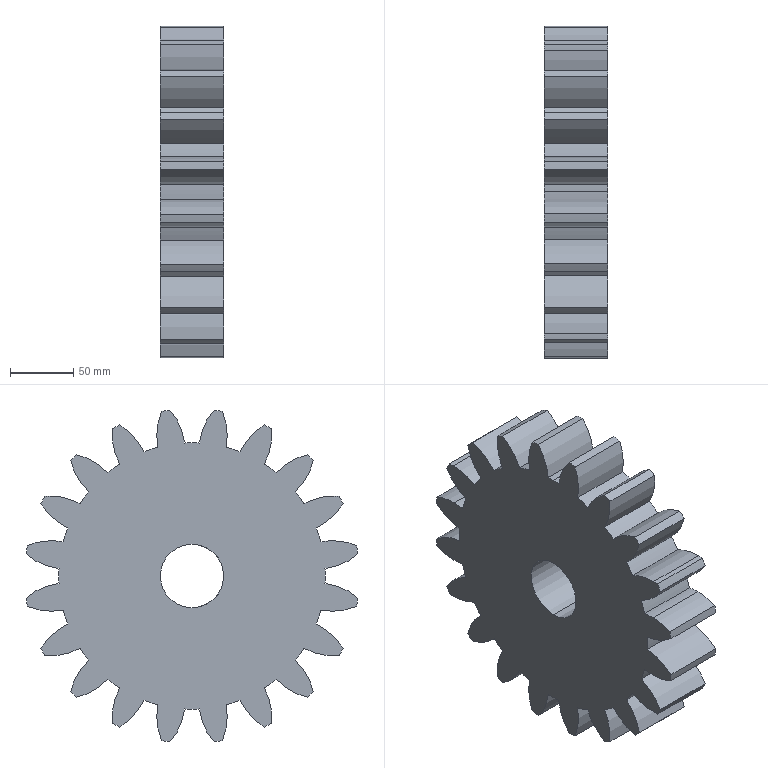Part | SolidWorks | features BaseBody 1, ICE 1 | 1 solid | 93 faces | box 50 x 261.706 x 261.706 mm | volume 2092246 mm3 | cylinder 87 | plane 6 | commonest cylinder face diameters 96 x44 209.998 x21 264 x20 50 x2